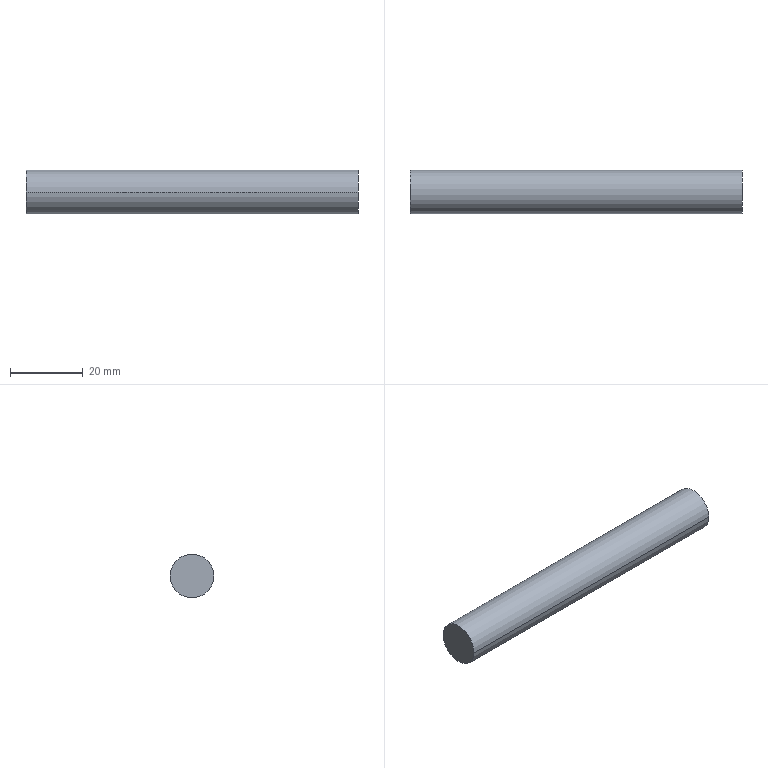Part | SolidWorks | features BaseBody 1 | 1 solid | 4 faces | box 90.963 x 12 x 12 mm | volume 10288 mm3 | plane 2 | cylinder 2 | commonest cylinder face diameters 12 x2
STEP:
#1=CARTESIAN_POINT('',(-619.405,438.283,590.465));
#2=VERTEX_POINT('',#1);
#3=CARTESIAN_POINT('',(-619.405,426.283,590.465));
#4=VERTEX_POINT('',#3);
#5=CARTESIAN_POINT('',(-619.405,432.283,590.465));
#6=DIRECTION('',(1.,0.,0.));
#7=DIRECTION('',(0.,1.,0.));
#8=AXIS2_PLACEMENT_3D('',#5,#6,#7);
#9=CIRCLE('',#8,6.);
#10=EDGE_CURVE('',#2,#4,#9,.T.);
#11=ORIENTED_EDGE('',*,*,#10,.F.);
#12=CARTESIAN_POINT('',(-619.405,432.283,590.465));
#13=DIRECTION('',(1.,0.,0.));
#14=DIRECTION('',(0.,1.,0.));
#15=AXIS2_PLACEMENT_3D('',#12,#13,#14);
#16=CIRCLE('',#15,6.);
#17=EDGE_CURVE('',#4,#2,#16,.T.);
#18=ORIENTED_EDGE('',*,*,#17,.F.);
#19=EDGE_LOOP('',(#11,#18));
#20=FACE_OUTER_BOUND('',#19,.T.);
#21=CARTESIAN_POINT('',(-619.405,432.283,590.465));
#22=DIRECTION('',(-1.,0.,0.));
#23=DIRECTION('',(0.,0.,1.));
#24=AXIS2_PLACEMENT_3D('',#21,#22,#23);
#25=PLANE('',#24);
#26=ADVANCED_FACE('',(#20),#25,.T.);
#27=CARTESIAN_POINT('',(-528.442,438.283,590.465));
#28=VERTEX_POINT('',#27);
#29=CARTESIAN_POINT('',(-528.442,426.283,590.465));
#30=VERTEX_POINT('',#29);
#31=CARTESIAN_POINT('',(-528.442,432.283,590.465));
#32=DIRECTION('',(-1.,0.,0.));
#33=DIRECTION('',(0.,1.,0.));
#34=AXIS2_PLACEMENT_3D('',#31,#32,#33);
#35=CIRCLE('',#34,6.);
#36=EDGE_CURVE('',#28,#30,#35,.T.);
#37=ORIENTED_EDGE('',*,*,#36,.F.);
#38=CARTESIAN_POINT('',(-528.442,432.283,590.465));
#39=DIRECTION('',(-1.,0.,0.));
#40=DIRECTION('',(0.,1.,0.));
#41=AXIS2_PLACEMENT_3D('',#38,#39,#40);
#42=CIRCLE('',#41,6.);
#43=EDGE_CURVE('',#30,#28,#42,.T.);
#44=ORIENTED_EDGE('',*,*,#43,.F.);
#45=EDGE_LOOP('',(#37,#44));
#46=FACE_OUTER_BOUND('',#45,.T.);
#47=CARTESIAN_POINT('',(-528.442,432.283,590.465));
#48=DIRECTION('',(-1.,0.,0.));
#49=DIRECTION('',(0.,0.,1.));
#50=AXIS2_PLACEMENT_3D('',#47,#48,#49);
#51=PLANE('',#50);
#52=ADVANCED_FACE('',(#46),#51,.F.);
#53=CARTESIAN_POINT('',(-619.405,426.283,590.465));
#54=DIRECTION('',(1.,0.,0.));
#55=VECTOR('',#54,1000.);
#56=LINE('',#53,#55);
#57=EDGE_CURVE('',#4,#30,#56,.T.);
#58=ORIENTED_EDGE('',*,*,#57,.F.);
#59=ORIENTED_EDGE('',*,*,#17,.T.);
#60=CARTESIAN_POINT('',(-619.405,438.283,590.465));
#61=DIRECTION('',(1.,0.,0.));
#62=VECTOR('',#61,1000.);
#63=LINE('',#60,#62);
#64=EDGE_CURVE('',#2,#28,#63,.T.);
#65=ORIENTED_EDGE('',*,*,#64,.T.);
#66=ORIENTED_EDGE('',*,*,#36,.T.);
#67=EDGE_LOOP('',(#58,#59,#65,#66));
#68=FACE_OUTER_BOUND('',#67,.T.);
#69=CARTESIAN_POINT('',(-619.405,432.283,590.465));
#70=DIRECTION('',(1.,0.,0.));
#71=DIRECTION('',(0.,1.,0.));
#72=AXIS2_PLACEMENT_3D('',#69,#70,#71);
#73=CYLINDRICAL_SURFACE('',#72,6.);
#74=ADVANCED_FACE('',(#68),#73,.T.);
#75=ORIENTED_EDGE('',*,*,#10,.T.);
#76=ORIENTED_EDGE('',*,*,#57,.T.);
#77=ORIENTED_EDGE('',*,*,#43,.T.);
#78=ORIENTED_EDGE('',*,*,#64,.F.);
#79=EDGE_LOOP('',(#75,#76,#77,#78));
#80=FACE_OUTER_BOUND('',#79,.T.);
#81=CARTESIAN_POINT('',(-619.405,432.283,590.465));
#82=DIRECTION('',(1.,0.,0.));
#83=DIRECTION('',(0.,1.,0.));
#84=AXIS2_PLACEMENT_3D('',#81,#82,#83);
#85=CYLINDRICAL_SURFACE('',#84,6.);
#86=ADVANCED_FACE('',(#80),#85,.T.);
#87=CLOSED_SHELL('',(#26,#52,#74,#86));
#88=MANIFOLD_SOLID_BREP('',#87);
#89=CARTESIAN_POINT('',(0.,0.,0.));
#90=DIRECTION('',(0.,0.,1.));
#91=DIRECTION('',(1.,0.,0.));
#92=AXIS2_PLACEMENT_3D('',#89,#90,#91);
#93=(LENGTH_UNIT()NAMED_UNIT(*)SI_UNIT(.MILLI.,.METRE.));
#94=UNCERTAINTY_MEASURE_WITH_UNIT(LENGTH_MEASURE(0.00001),#93,'','');
#95=(NAMED_UNIT(*)PLANE_ANGLE_UNIT()SI_UNIT($,.RADIAN.));
#96=(NAMED_UNIT(*)SI_UNIT($,.STERADIAN.)SOLID_ANGLE_UNIT());
#97=(GEOMETRIC_REPRESENTATION_CONTEXT(3)GLOBAL_UNCERTAINTY_ASSIGNED_CONTEXT((#94))GLOBAL_UNIT_ASSIGNED_CONTEXT((#93,#95,#96))REPRESENTATION_CONTEXT('',''));
#98=ADVANCED_BREP_SHAPE_REPRESENTATION('',(#88,#92),#97);